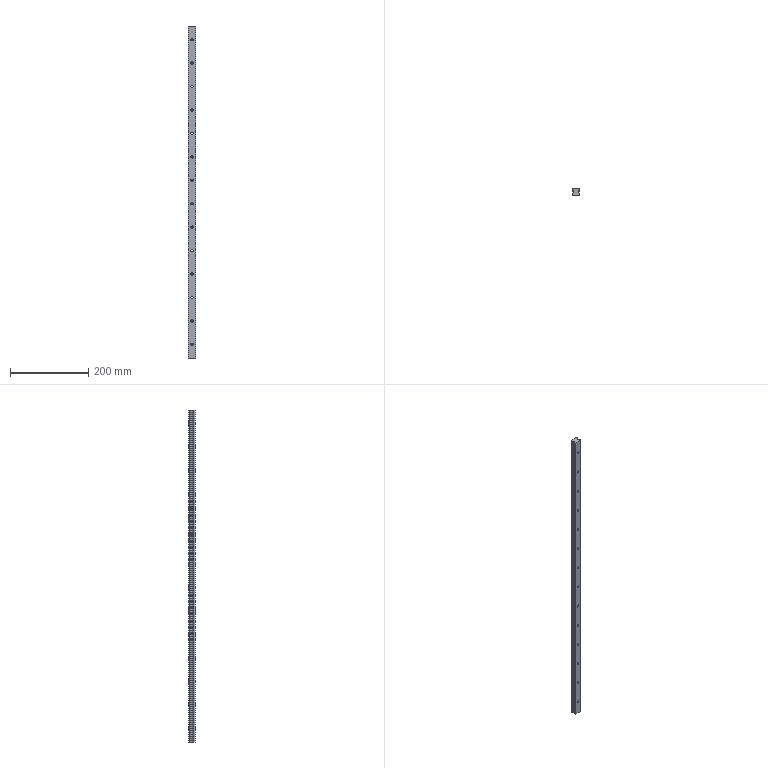Part | STEP file | C-HLGHA20-850_r | 1 solid | 86 faces | box 20 x 17.5 x 850 mm | volume 242038 mm3 | cylinder 50 | plane 36 | commonest cylinder face diameters 6 x14 9.5 x14 1 x12 2 x6 4.06 x4